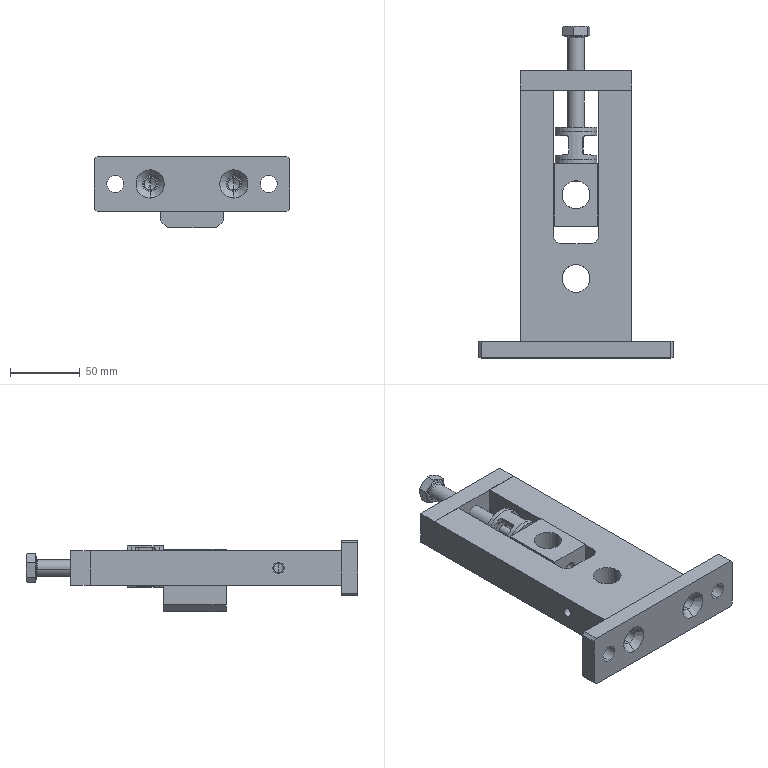Part | SolidWorks | features AEMSimFeature 1 | 5 solids | 168 faces | box 140 x 238 x 51.5 mm | volume 422457 mm3 | cylinder 74 | plane 70 | cone 22 | torus 2 | commonest cylinder face diameters 10 x10 12 x10 4 x8 8.5 x8 11 x8 6.8 x6